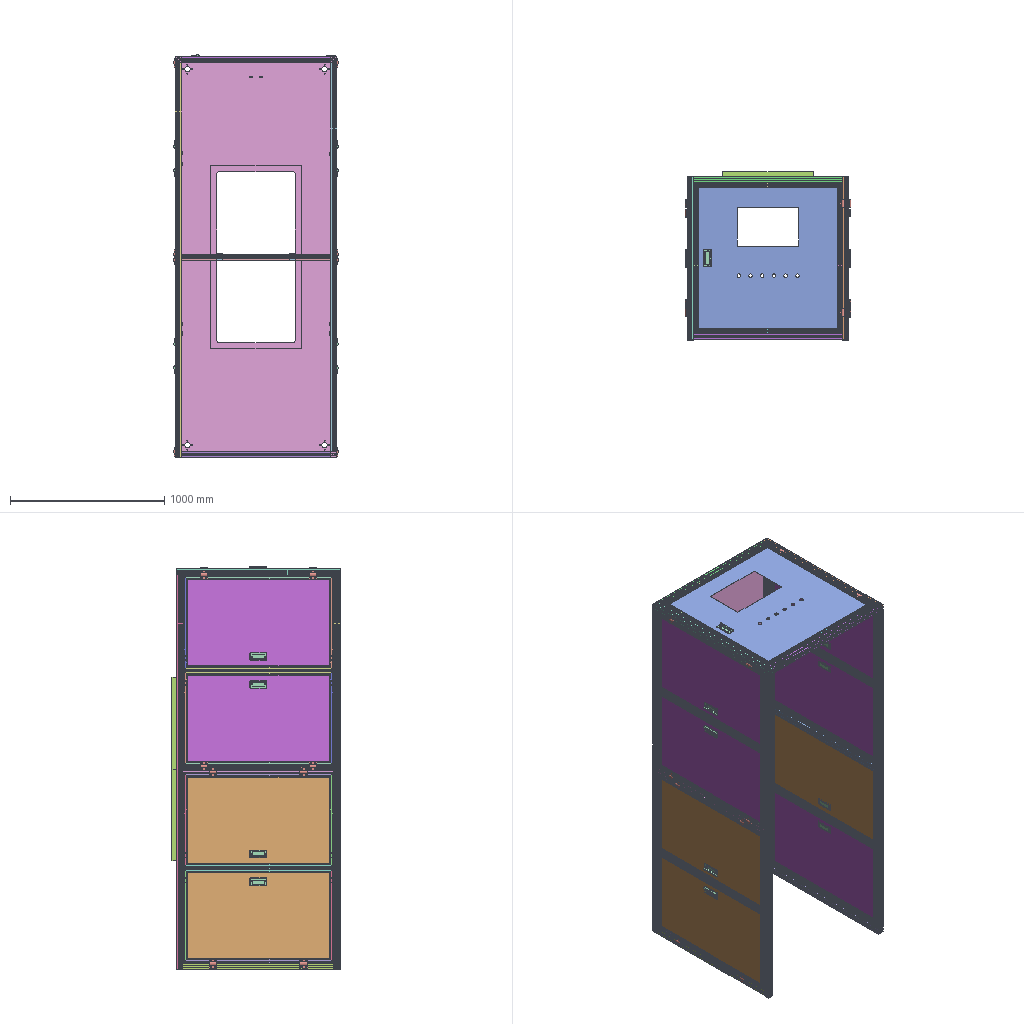Assembly | SolidWorks | 20 different items | 62 placed | box 1072 x 1092 x 2615 mm
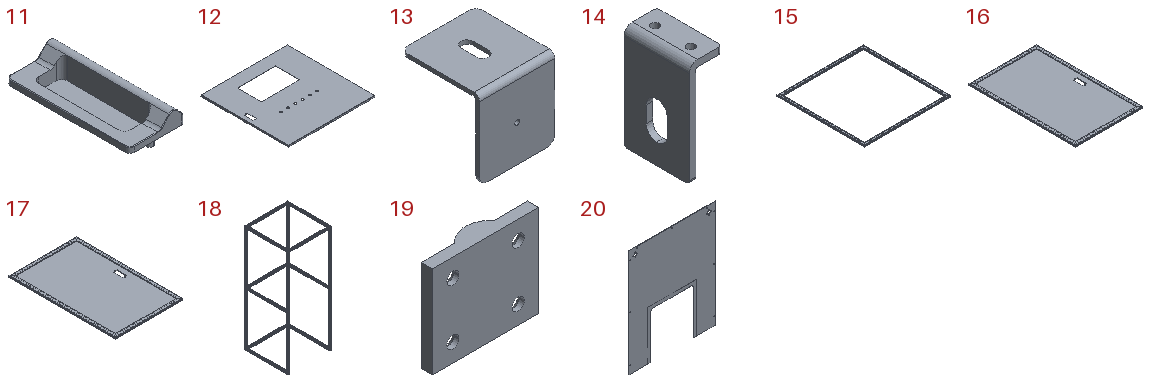Parts list (item | name | quantity | size | volume | features):
1 | AA1805NO | x1 | - | - | -
2 | AAD018-2-B-24V | x1 | - | - | -
3 | AAK-WB15.6 inch appearance only3D | x1 | - | - | -
4 | AAYW1B-V4E01R emergency stop | x1 | - | - | -
5 | AAYW1L-MF2E10Q4G(24V green) | x1 | - | - | -
6 | AAYW1L-MF2E10Q4R(24V red) | x1 | - | - | -
7 | AAYW1L-MF2E10Q4Y(24V yellow) | x1 | - | - | -
8 | AAZHC31-B emergency stop guard base | x1 | - | - | -
9 | AAZHE77-600-1 fluorescent lamp | x1 | - | - | -
10 | AA2-in-1 power switch φ22 H | x1 | - | - | -
11 | - | x9 | 50 x 110 x 23 mm | 40280 mm3 | features BaseBody 1
12 | - | x1 | 905 x 915 x 15 mm | 1150481 mm3 | features ICE 5, EdgeFlange 1, FlatPattern 1, LPattern 1, SMBaseFlange 1, SheetMetal 1
13 | - | x2 | 40 x 42 x 42 mm | 6284 mm3 | features EdgeFlange 1, Fillet 1, FlatPattern 1, HoleWzd 1, ICE 1, SMBaseFlange 1, SheetMetal 1
14 | - | x10 | 10 x 20 x 32 mm | 1421 mm3 | features BaseBody 1, HoleWzd 1
15 | - | x1 | 967 x 978 x 15 mm | 980488 mm3 | features WeldCornerFeat 4, HoleWzd 2, 3DProfileFeature 1, WeldMemberFeat 1, WeldmentFeature 1
16 | - | x5 | 618.5 x 978 x 15 mm | 4035765 mm3 | features WeldCornerFeat 4, HoleWzd 2, ICE 2, 3DProfileFeature 1, WeldMemberFeat 1, WeldmentFeature 1
17 | - | x3 | 618.5 x 978 x 15 mm | 4035765 mm3 | features WeldCornerFeat 4, HoleWzd 2, ICE 2, 3DProfileFeature 1, WeldMemberFeat 1, WeldmentFeature 1
18 | - | x1 | 1050 x 1060 x 2600 mm | 7986289 mm3 | features WeldCornerFeat 3, 3DProfileFeature 1, HoleWzd 1, WeldMemberFeat 1, WeldmentFeature 1
19 | - | x18 | 58 x 11 x 50 mm | 19652 mm3 | features BaseBody 1
20 | - | x2 | 1050 x 31.5 x 1300 mm | 1699042 mm3 | features Fillet 2, FlatPattern 2, ICE 2, SMBaseFlange 2, SheetMetal 2, Cut 1, MirrorPattern 1
Mates (type | each side: item.copy, entity, surface, feature):
Concentric | 17.1 face cylinder M6 Tapped Hole1 | 19.1 face cylinder Imported1 | 4 times
Concentric | 17.1 face cylinder M6 Tapped Hole1 | 19.2 face cylinder Imported1 | 2 times
Coincident | 17.1 face plane Aluminum profile 1530(1) | 19.2 face plane Imported1
Concentric | 17.1 face cylinder Cut-Extrude1 | 11.1 face cylinder Imported1 | 2 times
Coincident | 17.1 face plane Boss-Extrude1 | 11.1 face plane Imported1
Coincident | 17.1 face plane Aluminum profile 1530(1) | 19.1 face plane Imported1
Coincident | 16.1 face plane Aluminum profile 1530(1) | 19.3 face plane Imported1
Concentric | 16.1 face cylinder M6 Tapped Hole1 | 19.3 face cylinder Imported1 | 2 times
Concentric | 16.1 face cylinder M6 Tapped Hole1 | 19.4 face cylinder Imported1 | 2 times
Coincident | 16.1 face plane Aluminum profile 1530(1) | 19.4 face plane Imported1
Concentric | 16.2 face cylinder M6 Tapped Hole1 | 19.5 face cylinder Imported1 | 2 times
Concentric | 16.2 face cylinder M6 Tapped Hole1 | 19.6 face cylinder Imported1 | 2 times
Coincident | 16.2 face plane Aluminum profile 1530(1) | 19.6 face plane Imported1
Coincident | 16.2 face plane Aluminum profile 1530(1) | 19.5 face plane Imported1
Concentric | 11.2 face cylinder Imported1 | 16.1 face cylinder Cut-Extrude1 | 2 times
Coincident | 11.2 face plane Imported1 | 16.1 face plane Boss-Extrude1
Concentric | 16.2 face cylinder Cut-Extrude1 | 11.3 face cylinder Imported1 | 2 times
Coincident | 16.2 face plane Boss-Extrude1 | 11.3 face plane Imported1
Coincident | 17.1 face plane Aluminum profile 1530(1) | 16.1 face plane Aluminum profile 1530(1) | 2 times
DistanceDim | 16.1 face plane Aluminum profile 1530(1) | 17.1 face plane Aluminum profile 1530(1)
Coincident | 16.2 face plane Aluminum profile 1530(1) | 16.1 face plane Aluminum profile 1530(1) | 2 times
DistanceDim | 16.2 face plane Aluminum profile 1530(1) | 16.1 face plane Aluminum profile 1530(1)
Coincident | 16.2 face plane Aluminum profile 1530(1) | 18.1 face plane 40 X 40A X R0.5 - Missing(1)
DistanceDim | 18.1 face plane 40 X 40A X R0.5 - Missing(1) | 16.2 face plane Aluminum profile 1530(1)
DistanceDim | 16.2 face plane Aluminum profile 1530(1) | 18.1 face plane 40 X 40A X R0.5 - Missing(1)
Concentric | 11.4 face cylinder Imported1 | 16.3 face cylinder Cut-Extrude1 | 2 times
Coincident | 11.4 face plane Imported1 | 16.3 face plane Boss-Extrude1
Concentric | 16.4 face cylinder Cut-Extrude1 | 11.5 face cylinder Imported1 | 2 times
Concentric | 16.3 face cylinder M6 Tapped Hole1 | 19.7 face cylinder Imported1 | 2 times
Coincident | 16.3 face plane Aluminum profile 1530(1) | 19.7 face plane Imported1
Concentric | 16.3 face cylinder M6 Tapped Hole1 | 19.8 face cylinder Imported1 | 2 times
Coincident | 16.3 face plane Aluminum profile 1530(1) | 19.8 face plane Imported1
Concentric | 19.9 face cylinder Imported1 | 16.4 face cylinder M6 Tapped Hole1 | 2 times
Coincident | 19.9 face plane Imported1 | 16.4 face plane Aluminum profile 1530(1)
Concentric | 16.4 face cylinder M6 Tapped Hole1 | 19.10 face cylinder Imported1 | 2 times
Coincident | 16.4 face plane Aluminum profile 1530(1) | 19.10 face plane Imported1
Coincident | 16.3 face plane Aluminum profile 1530(1) | 16.4 face plane Aluminum profile 1530(1) | 2 times
DistanceDim | 16.4 face plane Aluminum profile 1530(1) | 16.3 face plane Aluminum profile 1530(1)
Coincident | 18.1 face plane 40 X 40A X R0.5 - Missing(1) | 16.4 face plane Aluminum profile 1530(1)
DistanceDim | 16.4 face plane Aluminum profile 1530(1) | 18.1 face plane 40 X 40A X R0.5 - Missing(1) | 2 times
Coincident | 16.4 face plane Boss-Extrude1 | 11.5 face plane Imported1
DistanceDim | 17.2 face plane Aluminum profile 1530(1) | 16.4 face plane Aluminum profile 1530(1)
Concentric | 17.2 face cylinder M6 Tapped Hole1 | 19.11 face cylinder Imported1 | 2 times
Concentric | 17.2 face cylinder M6 Tapped Hole1 | 19.12 face cylinder Imported1 | 2 times
Coincident | 20.1 face plane Base-Flange1 | 20.2 face plane Base-Flange1 | 2 times
Coincident | 16.4 face plane Aluminum profile 1530(1) | 17.2 face plane Aluminum profile 1530(1) | 2 times
Coincident | 17.2 face plane Aluminum profile 1530(1) | 19.12 face plane Imported1
Coincident | 17.2 face plane Aluminum profile 1530(1) | 19.11 face plane Imported1
Concentric | 17.2 face cylinder Cut-Extrude1 | 11.6 face cylinder Imported1 | 2 times
Coincident | 17.2 face plane Boss-Extrude1 | 11.6 face plane Imported1
Coincident | 15.1 face plane Aluminum profile 1530(1) | 12.1 face plane Base-Flange1
DistanceDim | 15.1 face plane Aluminum profile 1530(1) | 12.1 face plane Edge-Flange1
DistanceDim | 12.1 face plane Edge-Flange1 | 15.1 face plane Aluminum profile 1530(1)
Concentric | 15.1 face cylinder M6 Tapped Hole1 | 19.13 face cylinder Imported1 | 2 times
Coincident | 15.1 face plane Aluminum profile 1530(1) | 19.13 face plane Imported1
Concentric | 15.1 face cylinder M6 Tapped Hole1 | 19.14 face cylinder Imported1 | 2 times
Coincident | 15.1 face plane Aluminum profile 1530(1) | 19.14 face plane Imported1
Coincident | 15.1 face plane Aluminum profile 1530(1) | 18.1 face plane 40 X 40A X R0.5 - Missing(1)
DistanceDim | 18.1 face plane 40 X 40A X R0.5 - Missing(1) | 15.1 face plane Aluminum profile 1530(1)
DistanceDim | 15.1 face plane Aluminum profile 1530(1) | 18.1 face plane 40 X 40A X R0.5 - Missing(1)
Parallel | assembly face | assembly face
Concentric | assembly face | assembly face
DistanceDim | assembly face | assembly face
Coincident | assembly face | assembly face | 3 times
Coincident | 13.1 face plane Base-Flange1 | 13.2 face plane Base-Flange1 | 2 times
Coincident | 18.1 face plane 40 X 40A X R0.5 - Missing(1) | 13.1 face plane Edge-Flange1 | 2 times
Coincident | 14.1 face plane Imported1 | 18.1 face plane 40 X 40A X R0.5 - Missing(1)
Coincident | 14.2 face plane Imported1 | 18.1 face plane 40 X 40A X R0.5 - Missing(1)
Coincident | 14.3 face plane Imported1 | 18.1 face plane 40 X 40A X R0.5 - Missing(1)
Coincident | 20.1 face plane Base-Flange1 | 18.1 face plane Trim/Extend3
Coincident | 20.1 face plane Base-Flange1 | 18.1 face plane 40 X 40A X R0.5 - Missing(1)
DistanceDim | 18.1 face plane 40 X 40A X R0.5 - Missing(1) | 20.1 face plane Base-Flange1
Coincident | 12.1 face plane Base-Flange1 | 11.7 face plane Imported1
Concentric | 12.1 face cylinder Cut-Extrude3 | 11.7 face cylinder Imported1
Parallel | 18.1 face plane 40 X 40A X R0.5 - Missing(1) | 11.7 face plane Imported1
Coincident | 11.8 face plane Imported1 | 17.3 face plane Boss-Extrude1
Coincident | 19.15 face plane Imported1 | 17.3 face plane Aluminum profile 1530(1)
Coincident | 19.16 face plane Imported1 | 17.3 face plane Aluminum profile 1530(1)
Concentric | 19.16 face cylinder Imported1 | 17.3 face cylinder M6 Tapped Hole1 | 4 times
Concentric | 11.8 face cylinder Imported1 | 17.3 face cylinder Cut-Extrude1 | 2 times
Concentric | 19.15 face cylinder Imported1 | 17.3 face cylinder M6 Tapped Hole1 | 2 times
Coincident | 18.1 face plane 40 X 40A X R0.5 - Missing(1) | 19.15 face plane Imported1
Coincident | 17.1 face plane Aluminum profile 1530(1) | 17.3 face plane Aluminum profile 1530(1)
DistanceDim | 17.3 face plane Aluminum profile 1530(1) | 18.1 face plane 40 X 40A X R0.5 - Missing(1)